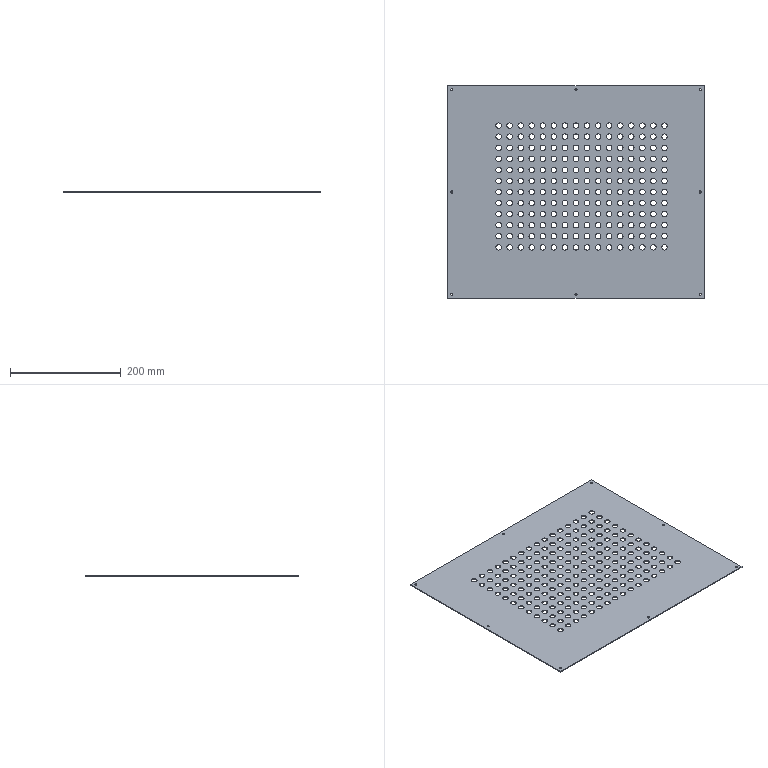Part | STEP file | x77-05302 | 1 solid | 406 faces | box 464 x 385 x 1.5 mm | volume 245190 mm3 | cylinder 400 | plane 6 | commonest cylinder face diameters 10 x384 4 x16